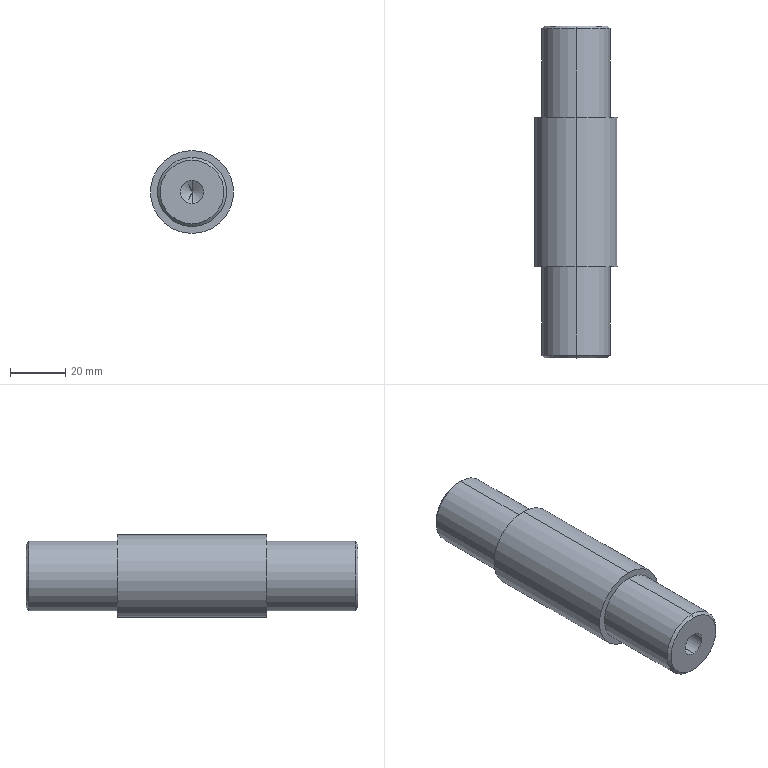Part | STEP file | PN_0023 | 1 solid | 22 faces | box 30 x 120 x 30 mm | volume 67614 mm3 | cylinder 10 | cone 8 | plane 4 | commonest cylinder face diameters 8.5 x4 25 x4 30 x2
STEP:
#1=CARTESIAN_POINT('',(0.,0.,0.));
#2=DIRECTION('',(0.,0.,1.));
#3=DIRECTION('',(1.,0.,0.));
#4=AXIS2_PLACEMENT_3D('',#1,#2,#3);
#5=CARTESIAN_POINT('',(0.,0.,-11.5));
#6=VERTEX_POINT('',#5);
#7=CARTESIAN_POINT('',(0.,0.,11.5));
#8=VERTEX_POINT('',#7);
#9=CARTESIAN_POINT('',(0.,0.,0.));
#10=DIRECTION('',(0.,-1.,0.));
#11=DIRECTION('',(0.,0.,-1.));
#12=AXIS2_PLACEMENT_3D('',#9,#10,#11);
#13=CIRCLE('',#12,11.5);
#14=CARTESIAN_POINT('',(0.,0.,0.));
#15=DIRECTION('',(0.,1.,0.));
#16=DIRECTION('',(0.,0.,1.));
#17=AXIS2_PLACEMENT_3D('',#14,#15,#16);
#18=CONICAL_SURFACE('',#17,11.5,0.7854);
#19=CARTESIAN_POINT('',(3.142,0.));
#20=DIRECTION('',(-1.,0.));
#21=VECTOR('',#20,1.);
#22=LINE('',#19,#21);
#23=(GEOMETRIC_REPRESENTATION_CONTEXT(2)PARAMETRIC_REPRESENTATION_CONTEXT()REPRESENTATION_CONTEXT('',''));
#24=DEFINITIONAL_REPRESENTATION('',(#22),#23);
#25=PCURVE('',#18,#24);
#26=CARTESIAN_POINT('',(0.,0.,0.));
#27=DIRECTION('',(0.,-1.,0.));
#28=DIRECTION('',(0.,0.,-1.));
#29=AXIS2_PLACEMENT_3D('',#26,#27,#28);
#30=PLANE('',#29);
#31=CARTESIAN_POINT('',(0.,0.));
#32=DIRECTION('',(1.,0.));
#33=AXIS2_PLACEMENT_2D('',#31,#32);
#34=CIRCLE('',#33,11.5);
#35=(GEOMETRIC_REPRESENTATION_CONTEXT(2)PARAMETRIC_REPRESENTATION_CONTEXT()REPRESENTATION_CONTEXT('',''));
#36=DEFINITIONAL_REPRESENTATION('',(#34),#35);
#37=PCURVE('',#30,#36);
#38=SURFACE_CURVE('',#13,(#25,#37),.PCURVE_S1.);
#39=EDGE_CURVE('',#6,#8,#38,.T.);
#40=ORIENTED_EDGE('',*,*,#39,.F.);
#41=CARTESIAN_POINT('',(0.,1.,-12.5));
#42=VERTEX_POINT('',#41);
#43=CARTESIAN_POINT('',(0.,0.,-11.5));
#44=DIRECTION('',(0.,0.7071,-0.7071));
#45=VECTOR('',#44,1.);
#46=LINE('',#43,#45);
#47=CARTESIAN_POINT('',(3.142,0.));
#48=DIRECTION('',(0.,1.));
#49=VECTOR('',#48,1.);
#50=LINE('',#47,#49);
#51=(GEOMETRIC_REPRESENTATION_CONTEXT(2)PARAMETRIC_REPRESENTATION_CONTEXT()REPRESENTATION_CONTEXT('',''));
#52=DEFINITIONAL_REPRESENTATION('',(#50),#51);
#53=PCURVE('',#18,#52);
#54=CARTESIAN_POINT('',(0.,0.,0.));
#55=DIRECTION('',(0.,1.,0.));
#56=DIRECTION('',(0.,0.,1.));
#57=AXIS2_PLACEMENT_3D('',#54,#55,#56);
#58=CONICAL_SURFACE('',#57,11.5,0.7854);
#59=CARTESIAN_POINT('',(3.142,0.));
#60=DIRECTION('',(0.,1.));
#61=VECTOR('',#60,1.);
#62=LINE('',#59,#61);
#63=(GEOMETRIC_REPRESENTATION_CONTEXT(2)PARAMETRIC_REPRESENTATION_CONTEXT()REPRESENTATION_CONTEXT('',''));
#64=DEFINITIONAL_REPRESENTATION('',(#62),#63);
#65=PCURVE('',#58,#64);
#66=SURFACE_CURVE('',#46,(#53,#65),.PCURVE_S1.);
#67=EDGE_CURVE('',#6,#42,#66,.T.);
#68=ORIENTED_EDGE('',*,*,#67,.T.);
#69=CARTESIAN_POINT('',(0.,1.,12.5));
#70=VERTEX_POINT('',#69);
#71=CARTESIAN_POINT('',(0.,1.,0.));
#72=DIRECTION('',(0.,1.,0.));
#73=DIRECTION('',(0.,0.,-1.));
#74=AXIS2_PLACEMENT_3D('',#71,#72,#73);
#75=CIRCLE('',#74,12.5);
#76=CARTESIAN_POINT('',(-3.142,1.));
#77=DIRECTION('',(1.,0.));
#78=VECTOR('',#77,1.);
#79=LINE('',#76,#78);
#80=(GEOMETRIC_REPRESENTATION_CONTEXT(2)PARAMETRIC_REPRESENTATION_CONTEXT()REPRESENTATION_CONTEXT('',''));
#81=DEFINITIONAL_REPRESENTATION('',(#79),#80);
#82=PCURVE('',#18,#81);
#83=CARTESIAN_POINT('',(0.,0.,0.));
#84=DIRECTION('',(0.,-1.,0.));
#85=DIRECTION('',(0.,0.,-1.));
#86=AXIS2_PLACEMENT_3D('',#83,#84,#85);
#87=CYLINDRICAL_SURFACE('',#86,12.5);
#88=CARTESIAN_POINT('',(6.283,-1.));
#89=DIRECTION('',(-1.,0.));
#90=VECTOR('',#89,1.);
#91=LINE('',#88,#90);
#92=(GEOMETRIC_REPRESENTATION_CONTEXT(2)PARAMETRIC_REPRESENTATION_CONTEXT()REPRESENTATION_CONTEXT('',''));
#93=DEFINITIONAL_REPRESENTATION('',(#91),#92);
#94=PCURVE('',#87,#93);
#95=SURFACE_CURVE('',#75,(#82,#94),.PCURVE_S1.);
#96=EDGE_CURVE('',#70,#42,#95,.T.);
#97=ORIENTED_EDGE('',*,*,#96,.F.);
#98=CARTESIAN_POINT('',(0.,0.,11.5));
#99=DIRECTION('',(0.,0.7071,0.7071));
#100=VECTOR('',#99,1.);
#101=LINE('',#98,#100);
#102=CARTESIAN_POINT('',(0.,0.));
#103=DIRECTION('',(0.,1.));
#104=VECTOR('',#103,1.);
#105=LINE('',#102,#104);
#106=(GEOMETRIC_REPRESENTATION_CONTEXT(2)PARAMETRIC_REPRESENTATION_CONTEXT()REPRESENTATION_CONTEXT('',''));
#107=DEFINITIONAL_REPRESENTATION('',(#105),#106);
#108=PCURVE('',#18,#107);
#109=CARTESIAN_POINT('',(6.283,0.));
#110=DIRECTION('',(0.,1.));
#111=VECTOR('',#110,1.);
#112=LINE('',#109,#111);
#113=(GEOMETRIC_REPRESENTATION_CONTEXT(2)PARAMETRIC_REPRESENTATION_CONTEXT()REPRESENTATION_CONTEXT('',''));
#114=DEFINITIONAL_REPRESENTATION('',(#112),#113);
#115=PCURVE('',#58,#114);
#116=SURFACE_CURVE('',#101,(#108,#115),.PCURVE_S1.);
#117=EDGE_CURVE('',#8,#70,#116,.T.);
#118=ORIENTED_EDGE('',*,*,#117,.F.);
#119=EDGE_LOOP('',(#40,#68,#97,#118));
#120=FACE_BOUND('',#119,.T.);
#121=ADVANCED_FACE('',(#120),#18,.T.);
#122=CARTESIAN_POINT('',(0.,120.,11.5));
#123=VERTEX_POINT('',#122);
#124=CARTESIAN_POINT('',(0.,120.,-11.5));
#125=VERTEX_POINT('',#124);
#126=CARTESIAN_POINT('',(0.,120.,0.));
#127=DIRECTION('',(0.,1.,0.));
#128=DIRECTION('',(0.,0.,1.));
#129=AXIS2_PLACEMENT_3D('',#126,#127,#128);
#130=CIRCLE('',#129,11.5);
#131=CARTESIAN_POINT('',(0.,119.,0.));
#132=DIRECTION('',(0.,-1.,0.));
#133=DIRECTION('',(0.,0.,-1.));
#134=AXIS2_PLACEMENT_3D('',#131,#132,#133);
#135=CONICAL_SURFACE('',#134,12.5,0.7854);
#136=CARTESIAN_POINT('',(3.142,-1.));
#137=DIRECTION('',(-1.,0.));
#138=VECTOR('',#137,1.);
#139=LINE('',#136,#138);
#140=(GEOMETRIC_REPRESENTATION_CONTEXT(2)PARAMETRIC_REPRESENTATION_CONTEXT()REPRESENTATION_CONTEXT('',''));
#141=DEFINITIONAL_REPRESENTATION('',(#139),#140);
#142=PCURVE('',#135,#141);
#143=CARTESIAN_POINT('',(0.,120.,0.));
#144=DIRECTION('',(0.,1.,0.));
#145=DIRECTION('',(0.,0.,1.));
#146=AXIS2_PLACEMENT_3D('',#143,#144,#145);
#147=PLANE('',#146);
#148=CARTESIAN_POINT('',(0.,0.));
#149=DIRECTION('',(1.,0.));
#150=AXIS2_PLACEMENT_2D('',#148,#149);
#151=CIRCLE('',#150,11.5);
#152=(GEOMETRIC_REPRESENTATION_CONTEXT(2)PARAMETRIC_REPRESENTATION_CONTEXT()REPRESENTATION_CONTEXT('',''));
#153=DEFINITIONAL_REPRESENTATION('',(#151),#152);
#154=PCURVE('',#147,#153);
#155=SURFACE_CURVE('',#130,(#142,#154),.PCURVE_S1.);
#156=EDGE_CURVE('',#123,#125,#155,.T.);
#157=ORIENTED_EDGE('',*,*,#156,.F.);
#158=CARTESIAN_POINT('',(0.,119.,12.5));
#159=VERTEX_POINT('',#158);
#160=CARTESIAN_POINT('',(0.,119.,12.5));
#161=DIRECTION('',(0.,-0.7071,0.7071));
#162=VECTOR('',#161,1.);
#163=LINE('',#160,#162);
#164=CARTESIAN_POINT('',(3.142,0.));
#165=DIRECTION('',(0.,1.));
#166=VECTOR('',#165,1.);
#167=LINE('',#164,#166);
#168=(GEOMETRIC_REPRESENTATION_CONTEXT(2)PARAMETRIC_REPRESENTATION_CONTEXT()REPRESENTATION_CONTEXT('',''));
#169=DEFINITIONAL_REPRESENTATION('',(#167),#168);
#170=PCURVE('',#135,#169);
#171=CARTESIAN_POINT('',(0.,119.,0.));
#172=DIRECTION('',(0.,-1.,0.));
#173=DIRECTION('',(0.,0.,-1.));
#174=AXIS2_PLACEMENT_3D('',#171,#172,#173);
#175=CONICAL_SURFACE('',#174,12.5,0.7854);
#176=CARTESIAN_POINT('',(3.142,0.));
#177=DIRECTION('',(0.,1.));
#178=VECTOR('',#177,1.);
#179=LINE('',#176,#178);
#180=(GEOMETRIC_REPRESENTATION_CONTEXT(2)PARAMETRIC_REPRESENTATION_CONTEXT()REPRESENTATION_CONTEXT('',''));
#181=DEFINITIONAL_REPRESENTATION('',(#179),#180);
#182=PCURVE('',#175,#181);
#183=SURFACE_CURVE('',#163,(#170,#182),.PCURVE_S1.);
#184=EDGE_CURVE('',#123,#159,#183,.T.);
#185=ORIENTED_EDGE('',*,*,#184,.T.);
#186=CARTESIAN_POINT('',(0.,119.,-12.5));
#187=VERTEX_POINT('',#186);
#188=CARTESIAN_POINT('',(0.,119.,0.));
#189=DIRECTION('',(0.,-1.,0.));
#190=DIRECTION('',(0.,0.,1.));
#191=AXIS2_PLACEMENT_3D('',#188,#189,#190);
#192=CIRCLE('',#191,12.5);
#193=CARTESIAN_POINT('',(-3.142,0.));
#194=DIRECTION('',(1.,0.));
#195=VECTOR('',#194,1.);
#196=LINE('',#193,#195);
#197=(GEOMETRIC_REPRESENTATION_CONTEXT(2)PARAMETRIC_REPRESENTATION_CONTEXT()REPRESENTATION_CONTEXT('',''));
#198=DEFINITIONAL_REPRESENTATION('',(#196),#197);
#199=PCURVE('',#135,#198);
#200=CARTESIAN_POINT('',(0.,0.,0.));
#201=DIRECTION('',(0.,-1.,0.));
#202=DIRECTION('',(0.,0.,-1.));
#203=AXIS2_PLACEMENT_3D('',#200,#201,#202);
#204=CYLINDRICAL_SURFACE('',#203,12.5);
#205=CARTESIAN_POINT('',(-3.142,-119.));
#206=DIRECTION('',(1.,0.));
#207=VECTOR('',#206,1.);
#208=LINE('',#205,#207);
#209=(GEOMETRIC_REPRESENTATION_CONTEXT(2)PARAMETRIC_REPRESENTATION_CONTEXT()REPRESENTATION_CONTEXT('',''));
#210=DEFINITIONAL_REPRESENTATION('',(#208),#209);
#211=PCURVE('',#204,#210);
#212=SURFACE_CURVE('',#192,(#199,#211),.PCURVE_S1.);
#213=EDGE_CURVE('',#187,#159,#212,.T.);
#214=ORIENTED_EDGE('',*,*,#213,.F.);
#215=CARTESIAN_POINT('',(0.,119.,-12.5));
#216=DIRECTION('',(0.,-0.7071,-0.7071));
#217=VECTOR('',#216,1.);
#218=LINE('',#215,#217);
#219=CARTESIAN_POINT('',(0.,0.));
#220=DIRECTION('',(0.,1.));
#221=VECTOR('',#220,1.);
#222=LINE('',#219,#221);
#223=(GEOMETRIC_REPRESENTATION_CONTEXT(2)PARAMETRIC_REPRESENTATION_CONTEXT()REPRESENTATION_CONTEXT('',''));
#224=DEFINITIONAL_REPRESENTATION('',(#222),#223);
#225=PCURVE('',#135,#224);
#226=CARTESIAN_POINT('',(6.283,0.));
#227=DIRECTION('',(0.,1.));
#228=VECTOR('',#227,1.);
#229=LINE('',#226,#228);
#230=(GEOMETRIC_REPRESENTATION_CONTEXT(2)PARAMETRIC_REPRESENTATION_CONTEXT()REPRESENTATION_CONTEXT('',''));
#231=DEFINITIONAL_REPRESENTATION('',(#229),#230);
#232=PCURVE('',#175,#231);
#233=SURFACE_CURVE('',#218,(#225,#232),.PCURVE_S1.);
#234=EDGE_CURVE('',#125,#187,#233,.T.);
#235=ORIENTED_EDGE('',*,*,#234,.F.);
#236=EDGE_LOOP('',(#157,#185,#214,#235));
#237=FACE_BOUND('',#236,.T.);
#238=ADVANCED_FACE('',(#237),#135,.T.);
#239=CARTESIAN_POINT('',(0.,24.5,-4.25));
#240=VERTEX_POINT('',#239);
#241=CARTESIAN_POINT('',(0.,0.,-4.25));
#242=VERTEX_POINT('',#241);
#243=CARTESIAN_POINT('',(0.,0.,-4.25));
#244=DIRECTION('',(0.,-1.,0.));
#245=VECTOR('',#244,1.);
#246=LINE('',#243,#245);
#247=CARTESIAN_POINT('',(0.,0.,0.));
#248=DIRECTION('',(0.,-1.,0.));
#249=DIRECTION('',(0.,0.,-1.));
#250=AXIS2_PLACEMENT_3D('',#247,#248,#249);
#251=CYLINDRICAL_SURFACE('',#250,4.25);
#252=CARTESIAN_POINT('',(6.283,0.));
#253=DIRECTION('',(0.,1.));
#254=VECTOR('',#253,1.);
#255=LINE('',#252,#254);
#256=(GEOMETRIC_REPRESENTATION_CONTEXT(2)PARAMETRIC_REPRESENTATION_CONTEXT()REPRESENTATION_CONTEXT('',''));
#257=DEFINITIONAL_REPRESENTATION('',(#255),#256);
#258=PCURVE('',#251,#257);
#259=CARTESIAN_POINT('',(0.,0.,0.));
#260=DIRECTION('',(0.,-1.,0.));
#261=DIRECTION('',(0.,0.,-1.));
#262=AXIS2_PLACEMENT_3D('',#259,#260,#261);
#263=CYLINDRICAL_SURFACE('',#262,4.25);
#264=CARTESIAN_POINT('',(0.,0.));
#265=DIRECTION('',(0.,1.));
#266=VECTOR('',#265,1.);
#267=LINE('',#264,#266);
#268=(GEOMETRIC_REPRESENTATION_CONTEXT(2)PARAMETRIC_REPRESENTATION_CONTEXT()REPRESENTATION_CONTEXT('',''));
#269=DEFINITIONAL_REPRESENTATION('',(#267),#268);
#270=PCURVE('',#263,#269);
#271=SURFACE_CURVE('',#246,(#258,#270),.PCURVE_S1.);
#272=EDGE_CURVE('',#240,#242,#271,.T.);
#273=ORIENTED_EDGE('',*,*,#272,.T.);
#274=CARTESIAN_POINT('',(0.,0.,4.25));
#275=VERTEX_POINT('',#274);
#276=CARTESIAN_POINT('',(0.,0.,0.));
#277=DIRECTION('',(0.,-1.,0.));
#278=DIRECTION('',(0.,0.,-1.));
#279=AXIS2_PLACEMENT_3D('',#276,#277,#278);
#280=CIRCLE('',#279,4.25);
#281=CARTESIAN_POINT('',(0.,0.));
#282=DIRECTION('',(1.,0.));
#283=VECTOR('',#282,1.);
#284=LINE('',#281,#283);
#285=(GEOMETRIC_REPRESENTATION_CONTEXT(2)PARAMETRIC_REPRESENTATION_CONTEXT()REPRESENTATION_CONTEXT('',''));
#286=DEFINITIONAL_REPRESENTATION('',(#284),#285);
#287=PCURVE('',#251,#286);
#288=CARTESIAN_POINT('',(0.,0.));
#289=DIRECTION('',(1.,0.));
#290=AXIS2_PLACEMENT_2D('',#288,#289);
#291=CIRCLE('',#290,4.25);
#292=(GEOMETRIC_REPRESENTATION_CONTEXT(2)PARAMETRIC_REPRESENTATION_CONTEXT()REPRESENTATION_CONTEXT('',''));
#293=DEFINITIONAL_REPRESENTATION('',(#291),#292);
#294=PCURVE('',#30,#293);
#295=SURFACE_CURVE('',#280,(#287,#294),.PCURVE_S1.);
#296=EDGE_CURVE('',#275,#242,#295,.T.);
#297=ORIENTED_EDGE('',*,*,#296,.F.);
#298=CARTESIAN_POINT('',(0.,24.5,4.25));
#299=VERTEX_POINT('',#298);
#300=CARTESIAN_POINT('',(0.,0.,4.25));
#301=DIRECTION('',(0.,-1.,0.));
#302=VECTOR('',#301,1.);
#303=LINE('',#300,#302);
#304=CARTESIAN_POINT('',(3.142,0.));
#305=DIRECTION('',(0.,1.));
#306=VECTOR('',#305,1.);
#307=LINE('',#304,#306);
#308=(GEOMETRIC_REPRESENTATION_CONTEXT(2)PARAMETRIC_REPRESENTATION_CONTEXT()REPRESENTATION_CONTEXT('',''));
#309=DEFINITIONAL_REPRESENTATION('',(#307),#308);
#310=PCURVE('',#251,#309);
#311=CARTESIAN_POINT('',(3.142,0.));
#312=DIRECTION('',(0.,1.));
#313=VECTOR('',#312,1.);
#314=LINE('',#311,#313);
#315=(GEOMETRIC_REPRESENTATION_CONTEXT(2)PARAMETRIC_REPRESENTATION_CONTEXT()REPRESENTATION_CONTEXT('',''));
#316=DEFINITIONAL_REPRESENTATION('',(#314),#315);
#317=PCURVE('',#263,#316);
#318=SURFACE_CURVE('',#303,(#310,#317),.PCURVE_S1.);
#319=EDGE_CURVE('',#299,#275,#318,.T.);
#320=ORIENTED_EDGE('',*,*,#319,.F.);
#321=CARTESIAN_POINT('',(0.,24.5,0.));
#322=DIRECTION('',(0.,-1.,0.));
#323=DIRECTION('',(0.,0.,-1.));
#324=AXIS2_PLACEMENT_3D('',#321,#322,#323);
#325=CIRCLE('',#324,4.25);
#326=CARTESIAN_POINT('',(0.,-24.5));
#327=DIRECTION('',(1.,0.));
#328=VECTOR('',#327,1.);
#329=LINE('',#326,#328);
#330=(GEOMETRIC_REPRESENTATION_CONTEXT(2)PARAMETRIC_REPRESENTATION_CONTEXT()REPRESENTATION_CONTEXT('',''));
#331=DEFINITIONAL_REPRESENTATION('',(#329),#330);
#332=PCURVE('',#251,#331);
#333=CARTESIAN_POINT('',(0.,24.5,0.));
#334=DIRECTION('',(0.,-1.,0.));
#335=DIRECTION('',(0.,0.,-1.));
#336=AXIS2_PLACEMENT_3D('',#333,#334,#335);
#337=CONICAL_SURFACE('',#336,4.25,1.03);
#338=CARTESIAN_POINT('',(0.,0.));
#339=DIRECTION('',(1.,0.));
#340=VECTOR('',#339,1.);
#341=LINE('',#338,#340);
#342=(GEOMETRIC_REPRESENTATION_CONTEXT(2)PARAMETRIC_REPRESENTATION_CONTEXT()REPRESENTATION_CONTEXT('',''));
#343=DEFINITIONAL_REPRESENTATION('',(#341),#342);
#344=PCURVE('',#337,#343);
#345=SURFACE_CURVE('',#325,(#332,#344),.PCURVE_S1.);
#346=EDGE_CURVE('',#299,#240,#345,.T.);
#347=ORIENTED_EDGE('',*,*,#346,.T.);
#348=EDGE_LOOP('',(#273,#297,#320,#347));
#349=FACE_BOUND('',#348,.F.);
#350=ADVANCED_FACE('',(#349),#251,.F.);
#351=ORIENTED_EDGE('',*,*,#346,.F.);
#352=CARTESIAN_POINT('',(0.,27.054,0.));
#353=VERTEX_POINT('',#352);
#354=CARTESIAN_POINT('',(0.,24.5,4.25));
#355=DIRECTION('',(0.,-0.515,0.8572));
#356=VECTOR('',#355,1.);
#357=LINE('',#354,#356);
#358=CARTESIAN_POINT('',(3.142,0.));
#359=DIRECTION('',(0.,1.));
#360=VECTOR('',#359,1.);
#361=LINE('',#358,#360);
#362=(GEOMETRIC_REPRESENTATION_CONTEXT(2)PARAMETRIC_REPRESENTATION_CONTEXT()REPRESENTATION_CONTEXT('',''));
#363=DEFINITIONAL_REPRESENTATION('',(#361),#362);
#364=PCURVE('',#337,#363);
#365=CARTESIAN_POINT('',(0.,24.5,0.));
#366=DIRECTION('',(0.,-1.,0.));
#367=DIRECTION('',(0.,0.,-1.));
#368=AXIS2_PLACEMENT_3D('',#365,#366,#367);
#369=CONICAL_SURFACE('',#368,4.25,1.03);
#370=CARTESIAN_POINT('',(3.142,0.));
#371=DIRECTION('',(0.,1.));
#372=VECTOR('',#371,1.);
#373=LINE('',#370,#372);
#374=(GEOMETRIC_REPRESENTATION_CONTEXT(2)PARAMETRIC_REPRESENTATION_CONTEXT()REPRESENTATION_CONTEXT('',''));
#375=DEFINITIONAL_REPRESENTATION('',(#373),#374);
#376=PCURVE('',#369,#375);
#377=SURFACE_CURVE('',#357,(#364,#376),.PCURVE_S1.);
#378=EDGE_CURVE('',#353,#299,#377,.T.);
#379=ORIENTED_EDGE('',*,*,#378,.F.);
#380=CARTESIAN_POINT('',(0.,24.5,-4.25));
#381=DIRECTION('',(0.,-0.515,-0.8572));
#382=VECTOR('',#381,1.);
#383=LINE('',#380,#382);
#384=CARTESIAN_POINT('',(6.283,0.));
#385=DIRECTION('',(0.,1.));
#386=VECTOR('',#385,1.);
#387=LINE('',#384,#386);
#388=(GEOMETRIC_REPRESENTATION_CONTEXT(2)PARAMETRIC_REPRESENTATION_CONTEXT()REPRESENTATION_CONTEXT('',''));
#389=DEFINITIONAL_REPRESENTATION('',(#387),#388);
#390=PCURVE('',#337,#389);
#391=CARTESIAN_POINT('',(0.,0.));
#392=DIRECTION('',(0.,1.));
#393=VECTOR('',#392,1.);
#394=LINE('',#391,#393);
#395=(GEOMETRIC_REPRESENTATION_CONTEXT(2)PARAMETRIC_REPRESENTATION_CONTEXT()REPRESENTATION_CONTEXT('',''));
#396=DEFINITIONAL_REPRESENTATION('',(#394),#395);
#397=PCURVE('',#369,#396);
#398=SURFACE_CURVE('',#383,(#390,#397),.PCURVE_S1.);
#399=EDGE_CURVE('',#353,#240,#398,.T.);
#400=ORIENTED_EDGE('',*,*,#399,.T.);
#401=EDGE_LOOP('',(#351,#379,#400));
#402=FACE_BOUND('',#401,.F.);
#403=ADVANCED_FACE('',(#402),#337,.F.);
#404=CARTESIAN_POINT('',(-0.002204,95.5,4.252));
#405=VERTEX_POINT('',#404);
#406=CARTESIAN_POINT('',(-0.002204,120.,4.252));
#407=VERTEX_POINT('',#406);
#408=CARTESIAN_POINT('',(-0.002204,120.,4.252));
#409=DIRECTION('',(0.,1.,0.));
#410=VECTOR('',#409,1.);
#411=LINE('',#408,#410);
#412=CARTESIAN_POINT('',(-0.002204,120.,0.001923));
#413=DIRECTION('',(0.,1.,0.));
#414=DIRECTION('',(0.,0.,1.));
#415=AXIS2_PLACEMENT_3D('',#412,#413,#414);
#416=CYLINDRICAL_SURFACE('',#415,4.25);
#417=CARTESIAN_POINT('',(6.283,0.));
#418=DIRECTION('',(0.,1.));
#419=VECTOR('',#418,1.);
#420=LINE('',#417,#419);
#421=(GEOMETRIC_REPRESENTATION_CONTEXT(2)PARAMETRIC_REPRESENTATION_CONTEXT()REPRESENTATION_CONTEXT('',''));
#422=DEFINITIONAL_REPRESENTATION('',(#420),#421);
#423=PCURVE('',#416,#422);
#424=CARTESIAN_POINT('',(-0.002204,120.,0.001923));
#425=DIRECTION('',(0.,1.,0.));
#426=DIRECTION('',(0.,0.,1.));
#427=AXIS2_PLACEMENT_3D('',#424,#425,#426);
#428=CYLINDRICAL_SURFACE('',#427,4.25);
#429=CARTESIAN_POINT('',(0.,0.));
#430=DIRECTION('',(0.,1.));
#431=VECTOR('',#430,1.);
#432=LINE('',#429,#431);
#433=(GEOMETRIC_REPRESENTATION_CONTEXT(2)PARAMETRIC_REPRESENTATION_CONTEXT()REPRESENTATION_CONTEXT('',''));
#434=DEFINITIONAL_REPRESENTATION('',(#432),#433);
#435=PCURVE('',#428,#434);
#436=SURFACE_CURVE('',#411,(#423,#435),.PCURVE_S1.);
#437=EDGE_CURVE('',#405,#407,#436,.T.);
#438=ORIENTED_EDGE('',*,*,#437,.T.);
#439=CARTESIAN_POINT('',(-0.002204,120.,-4.248));
#440=VERTEX_POINT('',#439);
#441=CARTESIAN_POINT('',(-0.002204,120.,0.001923));
#442=DIRECTION('',(0.,1.,0.));
#443=DIRECTION('',(0.,0.,1.));
#444=AXIS2_PLACEMENT_3D('',#441,#442,#443);
#445=CIRCLE('',#444,4.25);
#446=CARTESIAN_POINT('',(0.,0.));
#447=DIRECTION('',(1.,0.));
#448=VECTOR('',#447,1.);
#449=LINE('',#446,#448);
#450=(GEOMETRIC_REPRESENTATION_CONTEXT(2)PARAMETRIC_REPRESENTATION_CONTEXT()REPRESENTATION_CONTEXT('',''));
#451=DEFINITIONAL_REPRESENTATION('',(#449),#450);
#452=PCURVE('',#416,#451);
#453=CARTESIAN_POINT('',(0.001923,-0.002204));
#454=DIRECTION('',(1.,0.));
#455=AXIS2_PLACEMENT_2D('',#453,#454);
#456=CIRCLE('',#455,4.25);
#457=(GEOMETRIC_REPRESENTATION_CONTEXT(2)PARAMETRIC_REPRESENTATION_CONTEXT()REPRESENTATION_CONTEXT('',''));
#458=DEFINITIONAL_REPRESENTATION('',(#456),#457);
#459=PCURVE('',#147,#458);
#460=SURFACE_CURVE('',#445,(#452,#459),.PCURVE_S1.);
#461=EDGE_CURVE('',#440,#407,#460,.T.);
#462=ORIENTED_EDGE('',*,*,#461,.F.);
#463=CARTESIAN_POINT('',(-0.002204,95.5,-4.248));
#464=VERTEX_POINT('',#463);
#465=CARTESIAN_POINT('',(-0.002204,120.,-4.248));
#466=DIRECTION('',(0.,1.,0.));
#467=VECTOR('',#466,1.);
#468=LINE('',#465,#467);
#469=CARTESIAN_POINT('',(3.142,0.));
#470=DIRECTION('',(0.,1.));
#471=VECTOR('',#470,1.);
#472=LINE('',#469,#471);
#473=(GEOMETRIC_REPRESENTATION_CONTEXT(2)PARAMETRIC_REPRESENTATION_CONTEXT()REPRESENTATION_CONTEXT('',''));
#474=DEFINITIONAL_REPRESENTATION('',(#472),#473);
#475=PCURVE('',#416,#474);
#476=CARTESIAN_POINT('',(3.142,0.));
#477=DIRECTION('',(0.,1.));
#478=VECTOR('',#477,1.);
#479=LINE('',#476,#478);
#480=(GEOMETRIC_REPRESENTATION_CONTEXT(2)PARAMETRIC_REPRESENTATION_CONTEXT()REPRESENTATION_CONTEXT('',''));
#481=DEFINITIONAL_REPRESENTATION('',(#479),#480);
#482=PCURVE('',#428,#481);
#483=SURFACE_CURVE('',#468,(#475,#482),.PCURVE_S1.);
#484=EDGE_CURVE('',#464,#440,#483,.T.);
#485=ORIENTED_EDGE('',*,*,#484,.F.);
#486=CARTESIAN_POINT('',(-0.002204,95.5,0.001923));
#487=DIRECTION('',(0.,1.,0.));
#488=DIRECTION('',(0.,0.,1.));
#489=AXIS2_PLACEMENT_3D('',#486,#487,#488);
#490=CIRCLE('',#489,4.25);
#491=CARTESIAN_POINT('',(0.,-24.5));
#492=DIRECTION('',(1.,0.));
#493=VECTOR('',#492,1.);
#494=LINE('',#491,#493);
#495=(GEOMETRIC_REPRESENTATION_CONTEXT(2)PARAMETRIC_REPRESENTATION_CONTEXT()REPRESENTATION_CONTEXT('',''));
#496=DEFINITIONAL_REPRESENTATION('',(#494),#495);
#497=PCURVE('',#416,#496);
#498=CARTESIAN_POINT('',(-0.002204,95.5,0.001923));
#499=DIRECTION('',(0.,1.,0.));
#500=DIRECTION('',(0.,0.,1.));
#501=AXIS2_PLACEMENT_3D('',#498,#499,#500);
#502=CONICAL_SURFACE('',#501,4.25,1.03);
#503=CARTESIAN_POINT('',(0.,0.));
#504=DIRECTION('',(1.,0.));
#505=VECTOR('',#504,1.);
#506=LINE('',#503,#505);
#507=(GEOMETRIC_REPRESENTATION_CONTEXT(2)PARAMETRIC_REPRESENTATION_CONTEXT()REPRESENTATION_CONTEXT('',''));
#508=DEFINITIONAL_REPRESENTATION('',(#506),#507);
#509=PCURVE('',#502,#508);
#510=SURFACE_CURVE('',#490,(#497,#509),.PCURVE_S1.);
#511=EDGE_CURVE('',#464,#405,#510,.T.);
#512=ORIENTED_EDGE('',*,*,#511,.T.);
#513=EDGE_LOOP('',(#438,#462,#485,#512));
#514=FACE_BOUND('',#513,.F.);
#515=ADVANCED_FACE('',(#514),#416,.F.);
#516=ORIENTED_EDGE('',*,*,#511,.F.);
#517=CARTESIAN_POINT('',(-0.002204,92.946,0.001923));
#518=VERTEX_POINT('',#517);
#519=CARTESIAN_POINT('',(-0.002204,95.5,-4.248));
#520=DIRECTION('',(0.,0.515,-0.8572));
#521=VECTOR('',#520,1.);
#522=LINE('',#519,#521);
#523=CARTESIAN_POINT('',(3.142,0.));
#524=DIRECTION('',(0.,1.));
#525=VECTOR('',#524,1.);
#526=LINE('',#523,#525);
#527=(GEOMETRIC_REPRESENTATION_CONTEXT(2)PARAMETRIC_REPRESENTATION_CONTEXT()REPRESENTATION_CONTEXT('',''));
#528=DEFINITIONAL_REPRESENTATION('',(#526),#527);
#529=PCURVE('',#502,#528);
#530=CARTESIAN_POINT('',(-0.002204,95.5,0.001923));
#531=DIRECTION('',(0.,1.,0.));
#532=DIRECTION('',(0.,0.,1.));
#533=AXIS2_PLACEMENT_3D('',#530,#531,#532);
#534=CONICAL_SURFACE('',#533,4.25,1.03);
#535=CARTESIAN_POINT('',(3.142,0.));
#536=DIRECTION('',(0.,1.));
#537=VECTOR('',#536,1.);
#538=LINE('',#535,#537);
#539=(GEOMETRIC_REPRESENTATION_CONTEXT(2)PARAMETRIC_REPRESENTATION_CONTEXT()REPRESENTATION_CONTEXT('',''));
#540=DEFINITIONAL_REPRESENTATION('',(#538),#539);
#541=PCURVE('',#534,#540);
#542=SURFACE_CURVE('',#522,(#529,#541),.PCURVE_S1.);
#543=EDGE_CURVE('',#518,#464,#542,.T.);
#544=ORIENTED_EDGE('',*,*,#543,.F.);
#545=CARTESIAN_POINT('',(-0.002204,95.5,4.252));
#546=DIRECTION('',(0.,0.515,0.8572));
#547=VECTOR('',#546,1.);
#548=LINE('',#545,#547);
#549=CARTESIAN_POINT('',(6.283,0.));
#550=DIRECTION('',(0.,1.));
#551=VECTOR('',#550,1.);
#552=LINE('',#549,#551);
#553=(GEOMETRIC_REPRESENTATION_CONTEXT(2)PARAMETRIC_REPRESENTATION_CONTEXT()REPRESENTATION_CONTEXT('',''));
#554=DEFINITIONAL_REPRESENTATION('',(#552),#553);
#555=PCURVE('',#502,#554);
#556=CARTESIAN_POINT('',(0.,0.));
#557=DIRECTION('',(0.,1.));
#558=VECTOR('',#557,1.);
#559=LINE('',#556,#558);
#560=(GEOMETRIC_REPRESENTATION_CONTEXT(2)PARAMETRIC_REPRESENTATION_CONTEXT()REPRESENTATION_CONTEXT('',''));
#561=DEFINITIONAL_REPRESENTATION('',(#559),#560);
#562=PCURVE('',#534,#561);
#563=SURFACE_CURVE('',#548,(#555,#562),.PCURVE_S1.);
#564=EDGE_CURVE('',#518,#405,#563,.T.);
#565=ORIENTED_EDGE('',*,*,#564,.T.);
#566=EDGE_LOOP('',(#516,#544,#565));
#567=FACE_BOUND('',#566,.F.);
#568=ADVANCED_FACE('',(#567),#502,.F.);
#569=CARTESIAN_POINT('',(0.,33.,-12.5));
#570=VERTEX_POINT('',#569);
#571=CARTESIAN_POINT('',(0.,33.,12.5));
#572=VERTEX_POINT('',#571);
#573=CARTESIAN_POINT('',(0.,33.,0.));
#574=DIRECTION('',(0.,-1.,0.));
#575=DIRECTION('',(0.,0.,-1.));
#576=AXIS2_PLACEMENT_3D('',#573,#574,#575);
#577=CIRCLE('',#576,12.5);
#578=CARTESIAN_POINT('',(0.,-33.));
#579=DIRECTION('',(1.,0.));
#580=VECTOR('',#579,1.);
#581=LINE('',#578,#580);
#582=(GEOMETRIC_REPRESENTATION_CONTEXT(2)PARAMETRIC_REPRESENTATION_CONTEXT()REPRESENTATION_CONTEXT('',''));
#583=DEFINITIONAL_REPRESENTATION('',(#581),#582);
#584=PCURVE('',#87,#583);
#585=CARTESIAN_POINT('',(12.5,33.,0.));
#586=DIRECTION('',(0.,-1.,0.));
#587=DIRECTION('',(0.,0.,-1.));
#588=AXIS2_PLACEMENT_3D('',#585,#586,#587);
#589=PLANE('',#588);
#590=CARTESIAN_POINT('',(0.,-12.5));
#591=DIRECTION('',(1.,0.));
#592=AXIS2_PLACEMENT_2D('',#590,#591);
#593=CIRCLE('',#592,12.5);
#594=(GEOMETRIC_REPRESENTATION_CONTEXT(2)PARAMETRIC_REPRESENTATION_CONTEXT()REPRESENTATION_CONTEXT('',''));
#595=DEFINITIONAL_REPRESENTATION('',(#593),#594);
#596=PCURVE('',#589,#595);
#597=SURFACE_CURVE('',#577,(#584,#596),.PCURVE_S1.);
#598=EDGE_CURVE('',#570,#572,#597,.T.);
#599=ORIENTED_EDGE('',*,*,#598,.T.);
#600=CARTESIAN_POINT('',(0.,0.,12.5));
#601=DIRECTION('',(0.,-1.,0.));
#602=VECTOR('',#601,1.);
#603=LINE('',#600,#602);
#604=CARTESIAN_POINT('',(3.142,0.));
#605=DIRECTION('',(0.,1.));
#606=VECTOR('',#605,1.);
#607=LINE('',#604,#606);
#608=(GEOMETRIC_REPRESENTATION_CONTEXT(2)PARAMETRIC_REPRESENTATION_CONTEXT()REPRESENTATION_CONTEXT('',''));
#609=DEFINITIONAL_REPRESENTATION('',(#607),#608);
#610=PCURVE('',#87,#609);
#611=CARTESIAN_POINT('',(0.,0.,0.));
#612=DIRECTION('',(0.,-1.,0.));
#613=DIRECTION('',(0.,0.,-1.));
#614=AXIS2_PLACEMENT_3D('',#611,#612,#613);
#615=CYLINDRICAL_SURFACE('',#614,12.5);
#616=CARTESIAN_POINT('',(3.142,0.));
#617=DIRECTION('',(0.,1.));
#618=VECTOR('',#617,1.);
#619=LINE('',#616,#618);
#620=(GEOMETRIC_REPRESENTATION_CONTEXT(2)PARAMETRIC_REPRESENTATION_CONTEXT()REPRESENTATION_CONTEXT('',''));
#621=DEFINITIONAL_REPRESENTATION('',(#619),#620);
#622=PCURVE('',#615,#621);
#623=SURFACE_CURVE('',#603,(#610,#622),.PCURVE_S1.);
#624=EDGE_CURVE('',#572,#70,#623,.T.);
#625=ORIENTED_EDGE('',*,*,#624,.T.);
#626=ORIENTED_EDGE('',*,*,#96,.T.);
#627=CARTESIAN_POINT('',(0.,0.,-12.5));
#628=DIRECTION('',(0.,-1.,0.));
#629=VECTOR('',#628,1.);
#630=LINE('',#627,#629);
#631=CARTESIAN_POINT('',(0.,0.));
#632=DIRECTION('',(0.,1.));
#633=VECTOR('',#632,1.);
#634=LINE('',#631,#633);
#635=(GEOMETRIC_REPRESENTATION_CONTEXT(2)PARAMETRIC_REPRESENTATION_CONTEXT()REPRESENTATION_CONTEXT('',''));
#636=DEFINITIONAL_REPRESENTATION('',(#634),#635);
#637=PCURVE('',#87,#636);
#638=CARTESIAN_POINT('',(6.283,0.));
#639=DIRECTION('',(0.,1.));
#640=VECTOR('',#639,1.);
#641=LINE('',#638,#640);
#642=(GEOMETRIC_REPRESENTATION_CONTEXT(2)PARAMETRIC_REPRESENTATION_CONTEXT()REPRESENTATION_CONTEXT('',''));
#643=DEFINITIONAL_REPRESENTATION('',(#641),#642);
#644=PCURVE('',#615,#643);
#645=SURFACE_CURVE('',#630,(#637,#644),.PCURVE_S1.);
#646=EDGE_CURVE('',#570,#42,#645,.T.);
#647=ORIENTED_EDGE('',*,*,#646,.F.);
#648=EDGE_LOOP('',(#599,#625,#626,#647));
#649=FACE_BOUND('',#648,.T.);
#650=ADVANCED_FACE('',(#649),#87,.T.);
#651=CARTESIAN_POINT('',(0.,87.,-15.));
#652=VERTEX_POINT('',#651);
#653=CARTESIAN_POINT('',(0.,87.,15.));
#654=VERTEX_POINT('',#653);
#655=CARTESIAN_POINT('',(0.,87.,0.));
#656=DIRECTION('',(0.,-1.,0.));
#657=DIRECTION('',(0.,0.,-1.));
#658=AXIS2_PLACEMENT_3D('',#655,#656,#657);
#659=CIRCLE('',#658,15.);
#660=CARTESIAN_POINT('',(0.,0.,0.));
#661=DIRECTION('',(0.,-1.,0.));
#662=DIRECTION('',(0.,0.,-1.));
#663=AXIS2_PLACEMENT_3D('',#660,#661,#662);
#664=CYLINDRICAL_SURFACE('',#663,15.);
#665=CARTESIAN_POINT('',(0.,-87.));
#666=DIRECTION('',(1.,0.));
#667=VECTOR('',#666,1.);
#668=LINE('',#665,#667);
#669=(GEOMETRIC_REPRESENTATION_CONTEXT(2)PARAMETRIC_REPRESENTATION_CONTEXT()REPRESENTATION_CONTEXT('',''));
#670=DEFINITIONAL_REPRESENTATION('',(#668),#669);
#671=PCURVE('',#664,#670);
#672=CARTESIAN_POINT('',(12.5,87.,0.));
#673=DIRECTION('',(0.,1.,0.));
#674=DIRECTION('',(0.,0.,1.));
#675=AXIS2_PLACEMENT_3D('',#672,#673,#674);
#676=PLANE('',#675);
#677=CARTESIAN_POINT('',(-15.,-12.5));
#678=CARTESIAN_POINT('',(-15.,13.481));
#679=CARTESIAN_POINT('',(7.5,0.4904));
#680=CARTESIAN_POINT('',(30.,-12.5));
#681=CARTESIAN_POINT('',(7.5,-25.49));
#682=CARTESIAN_POINT('',(-15.,-38.481));
#683=CARTESIAN_POINT('',(-15.,-12.5));
#684=(BOUNDED_CURVE()B_SPLINE_CURVE(2,(#677,#678,#679,#680,#681,#682,#683),.UNSPECIFIED.,.T.,.F.)B_SPLINE_CURVE_WITH_KNOTS((1,2,2,2,2,1),(-2.094,0.,2.094,4.189,6.283,8.378),.UNSPECIFIED.)CURVE()GEOMETRIC_REPRESENTATION_ITEM()RATIONAL_B_SPLINE_CURVE((1.,0.5,1.,0.5,1.,0.5,1.))REPRESENTATION_ITEM(''));
#685=(GEOMETRIC_REPRESENTATION_CONTEXT(2)PARAMETRIC_REPRESENTATION_CONTEXT()REPRESENTATION_CONTEXT('',''));
#686=DEFINITIONAL_REPRESENTATION('',(#684),#685);
#687=PCURVE('',#676,#686);
#688=SURFACE_CURVE('',#659,(#671,#687),.PCURVE_S1.);
#689=EDGE_CURVE('',#652,#654,#688,.T.);
#690=ORIENTED_EDGE('',*,*,#689,.T.);
#691=CARTESIAN_POINT('',(0.,33.,15.));
#692=VERTEX_POINT('',#691);
#693=CARTESIAN_POINT('',(0.,0.,15.));
#694=DIRECTION('',(0.,-1.,0.));
#695=VECTOR('',#694,1.);
#696=LINE('',#693,#695);
#697=CARTESIAN_POINT('',(3.142,0.));
#698=DIRECTION('',(0.,1.));
#699=VECTOR('',#698,1.);
#700=LINE('',#697,#699);
#701=(GEOMETRIC_REPRESENTATION_CONTEXT(2)PARAMETRIC_REPRESENTATION_CONTEXT()REPRESENTATION_CONTEXT('',''));
#702=DEFINITIONAL_REPRESENTATION('',(#700),#701);
#703=PCURVE('',#664,#702);
#704=CARTESIAN_POINT('',(0.,0.,0.));
#705=DIRECTION('',(0.,-1.,0.));
#706=DIRECTION('',(0.,0.,-1.));
#707=AXIS2_PLACEMENT_3D('',#704,#705,#706);
#708=CYLINDRICAL_SURFACE('',#707,15.);
#709=CARTESIAN_POINT('',(3.142,0.));
#710=DIRECTION('',(0.,1.));
#711=VECTOR('',#710,1.);
#712=LINE('',#709,#711);
#713=(GEOMETRIC_REPRESENTATION_CONTEXT(2)PARAMETRIC_REPRESENTATION_CONTEXT()REPRESENTATION_CONTEXT('',''));
#714=DEFINITIONAL_REPRESENTATION('',(#712),#713);
#715=PCURVE('',#708,#714);
#716=SURFACE_CURVE('',#696,(#703,#715),.PCURVE_S1.);
#717=EDGE_CURVE('',#654,#692,#716,.T.);
#718=ORIENTED_EDGE('',*,*,#717,.T.);
#719=CARTESIAN_POINT('',(0.,33.,-15.));
#720=VERTEX_POINT('',#719);
#721=CARTESIAN_POINT('',(0.,33.,0.));
#722=DIRECTION('',(0.,-1.,0.));
#723=DIRECTION('',(0.,0.,-1.));
#724=AXIS2_PLACEMENT_3D('',#721,#722,#723);
#725=CIRCLE('',#724,15.);
#726=CARTESIAN_POINT('',(0.,-33.));
#727=DIRECTION('',(1.,0.));
#728=VECTOR('',#727,1.);
#729=LINE('',#726,#728);
#730=(GEOMETRIC_REPRESENTATION_CONTEXT(2)PARAMETRIC_REPRESENTATION_CONTEXT()REPRESENTATION_CONTEXT('',''));
#731=DEFINITIONAL_REPRESENTATION('',(#729),#730);
#732=PCURVE('',#664,#731);
#733=CARTESIAN_POINT('',(0.,-12.5));
#734=DIRECTION('',(1.,0.));
#735=AXIS2_PLACEMENT_2D('',#733,#734);
#736=CIRCLE('',#735,15.);
#737=(GEOMETRIC_REPRESENTATION_CONTEXT(2)PARAMETRIC_REPRESENTATION_CONTEXT()REPRESENTATION_CONTEXT('',''));
#738=DEFINITIONAL_REPRESENTATION('',(#736),#737);
#739=PCURVE('',#589,#738);
#740=SURFACE_CURVE('',#725,(#732,#739),.PCURVE_S1.);
#741=EDGE_CURVE('',#720,#692,#740,.T.);
#742=ORIENTED_EDGE('',*,*,#741,.F.);
#743=CARTESIAN_POINT('',(0.,0.,-15.));
#744=DIRECTION('',(0.,-1.,0.));
#745=VECTOR('',#744,1.);
#746=LINE('',#743,#745);
#747=CARTESIAN_POINT('',(0.,0.));
#748=DIRECTION('',(0.,1.));
#749=VECTOR('',#748,1.);
#750=LINE('',#747,#749);
#751=(GEOMETRIC_REPRESENTATION_CONTEXT(2)PARAMETRIC_REPRESENTATION_CONTEXT()REPRESENTATION_CONTEXT('',''));
#752=DEFINITIONAL_REPRESENTATION('',(#750),#751);
#753=PCURVE('',#664,#752);
#754=CARTESIAN_POINT('',(6.283,0.));
#755=DIRECTION('',(0.,1.));
#756=VECTOR('',#755,1.);
#757=LINE('',#754,#756);
#758=(GEOMETRIC_REPRESENTATION_CONTEXT(2)PARAMETRIC_REPRESENTATION_CONTEXT()REPRESENTATION_CONTEXT('',''));
#759=DEFINITIONAL_REPRESENTATION('',(#757),#758);
#760=PCURVE('',#708,#759);
#761=SURFACE_CURVE('',#746,(#753,#760),.PCURVE_S1.);
#762=EDGE_CURVE('',#652,#720,#761,.T.);
#763=ORIENTED_EDGE('',*,*,#762,.F.);
#764=EDGE_LOOP('',(#690,#718,#742,#763));
#765=FACE_BOUND('',#764,.T.);
#766=ADVANCED_FACE('',(#765),#664,.T.);
#767=ORIENTED_EDGE('',*,*,#213,.T.);
#768=CARTESIAN_POINT('',(0.,87.,12.5));
#769=VERTEX_POINT('',#768);
#770=CARTESIAN_POINT('',(0.,0.,12.5));
#771=DIRECTION('',(0.,-1.,0.));
#772=VECTOR('',#771,1.);
#773=LINE('',#770,#772);
#774=CARTESIAN_POINT('',(3.142,0.));
#775=DIRECTION('',(0.,1.));
#776=VECTOR('',#775,1.);
#777=LINE('',#774,#776);
#778=(GEOMETRIC_REPRESENTATION_CONTEXT(2)PARAMETRIC_REPRESENTATION_CONTEXT()REPRESENTATION_CONTEXT('',''));
#779=DEFINITIONAL_REPRESENTATION('',(#777),#778);
#780=PCURVE('',#204,#779);
#781=CARTESIAN_POINT('',(0.,0.,0.));
#782=DIRECTION('',(0.,-1.,0.));
#783=DIRECTION('',(0.,0.,-1.));
#784=AXIS2_PLACEMENT_3D('',#781,#782,#783);
#785=CYLINDRICAL_SURFACE('',#784,12.5);
#786=CARTESIAN_POINT('',(3.142,0.));
#787=DIRECTION('',(0.,1.));
#788=VECTOR('',#787,1.);
#789=LINE('',#786,#788);
#790=(GEOMETRIC_REPRESENTATION_CONTEXT(2)PARAMETRIC_REPRESENTATION_CONTEXT()REPRESENTATION_CONTEXT('',''));
#791=DEFINITIONAL_REPRESENTATION('',(#789),#790);
#792=PCURVE('',#785,#791);
#793=SURFACE_CURVE('',#773,(#780,#792),.PCURVE_S1.);
#794=EDGE_CURVE('',#159,#769,#793,.T.);
#795=ORIENTED_EDGE('',*,*,#794,.T.);
#796=CARTESIAN_POINT('',(0.,87.,-12.5));
#797=VERTEX_POINT('',#796);
#798=CARTESIAN_POINT('',(0.,87.,0.));
#799=DIRECTION('',(0.,-1.,0.));
#800=DIRECTION('',(0.,0.,-1.));
#801=AXIS2_PLACEMENT_3D('',#798,#799,#800);
#802=CIRCLE('',#801,12.5);
#803=CARTESIAN_POINT('',(0.,-87.));
#804=DIRECTION('',(1.,0.));
#805=VECTOR('',#804,1.);
#806=LINE('',#803,#805);
#807=(GEOMETRIC_REPRESENTATION_CONTEXT(2)PARAMETRIC_REPRESENTATION_CONTEXT()REPRESENTATION_CONTEXT('',''));
#808=DEFINITIONAL_REPRESENTATION('',(#806),#807);
#809=PCURVE('',#204,#808);
#810=CARTESIAN_POINT('',(-12.5,-12.5));
#811=CARTESIAN_POINT('',(-12.5,9.151));
#812=CARTESIAN_POINT('',(6.25,-1.675));
#813=CARTESIAN_POINT('',(25.,-12.5));
#814=CARTESIAN_POINT('',(6.25,-23.325));
#815=CARTESIAN_POINT('',(-12.5,-34.151));
#816=CARTESIAN_POINT('',(-12.5,-12.5));
#817=(BOUNDED_CURVE()B_SPLINE_CURVE(2,(#810,#811,#812,#813,#814,#815,#816),.UNSPECIFIED.,.T.,.F.)B_SPLINE_CURVE_WITH_KNOTS((1,2,2,2,2,1),(-2.094,0.,2.094,4.189,6.283,8.378),.UNSPECIFIED.)CURVE()GEOMETRIC_REPRESENTATION_ITEM()RATIONAL_B_SPLINE_CURVE((1.,0.5,1.,0.5,1.,0.5,1.))REPRESENTATION_ITEM(''));
#818=(GEOMETRIC_REPRESENTATION_CONTEXT(2)PARAMETRIC_REPRESENTATION_CONTEXT()REPRESENTATION_CONTEXT('',''));
#819=DEFINITIONAL_REPRESENTATION('',(#817),#818);
#820=PCURVE('',#676,#819);
#821=SURFACE_CURVE('',#802,(#809,#820),.PCURVE_S1.);
#822=EDGE_CURVE('',#797,#769,#821,.T.);
#823=ORIENTED_EDGE('',*,*,#822,.F.);
#824=CARTESIAN_POINT('',(0.,0.,-12.5));
#825=DIRECTION('',(0.,-1.,0.));
#826=VECTOR('',#825,1.);
#827=LINE('',#824,#826);
#828=CARTESIAN_POINT('',(0.,0.));
#829=DIRECTION('',(0.,1.));
#830=VECTOR('',#829,1.);
#831=LINE('',#828,#830);
#832=(GEOMETRIC_REPRESENTATION_CONTEXT(2)PARAMETRIC_REPRESENTATION_CONTEXT()REPRESENTATION_CONTEXT('',''));
#833=DEFINITIONAL_REPRESENTATION('',(#831),#832);
#834=PCURVE('',#204,#833);
#835=CARTESIAN_POINT('',(6.283,0.));
#836=DIRECTION('',(0.,1.));
#837=VECTOR('',#836,1.);
#838=LINE('',#835,#837);
#839=(GEOMETRIC_REPRESENTATION_CONTEXT(2)PARAMETRIC_REPRESENTATION_CONTEXT()REPRESENTATION_CONTEXT('',''));
#840=DEFINITIONAL_REPRESENTATION('',(#838),#839);
#841=PCURVE('',#785,#840);
#842=SURFACE_CURVE('',#827,(#834,#841),.PCURVE_S1.);
#843=EDGE_CURVE('',#187,#797,#842,.T.);
#844=ORIENTED_EDGE('',*,*,#843,.F.);
#845=EDGE_LOOP('',(#767,#795,#823,#844));
#846=FACE_BOUND('',#845,.T.);
#847=ADVANCED_FACE('',(#846),#204,.T.);
#848=CARTESIAN_POINT('',(0.,120.,0.));
#849=DIRECTION('',(0.,1.,0.));
#850=DIRECTION('',(0.,0.,1.));
#851=AXIS2_PLACEMENT_3D('',#848,#849,#850);
#852=CIRCLE('',#851,11.5);
#853=CARTESIAN_POINT('',(0.,0.));
#854=DIRECTION('',(1.,0.));
#855=AXIS2_PLACEMENT_2D('',#853,#854);
#856=CIRCLE('',#855,11.5);
#857=(GEOMETRIC_REPRESENTATION_CONTEXT(2)PARAMETRIC_REPRESENTATION_CONTEXT()REPRESENTATION_CONTEXT('',''));
#858=DEFINITIONAL_REPRESENTATION('',(#856),#857);
#859=PCURVE('',#147,#858);
#860=CARTESIAN_POINT('',(9.425,-1.));
#861=DIRECTION('',(-1.,0.));
#862=VECTOR('',#861,1.);
#863=LINE('',#860,#862);
#864=(GEOMETRIC_REPRESENTATION_CONTEXT(2)PARAMETRIC_REPRESENTATION_CONTEXT()REPRESENTATION_CONTEXT('',''));
#865=DEFINITIONAL_REPRESENTATION('',(#863),#864);
#866=PCURVE('',#175,#865);
#867=SURFACE_CURVE('',#852,(#859,#866),.PCURVE_S1.);
#868=EDGE_CURVE('',#125,#123,#867,.T.);
#869=ORIENTED_EDGE('',*,*,#868,.T.);
#870=ORIENTED_EDGE('',*,*,#156,.T.);
#871=EDGE_LOOP('',(#869,#870));
#872=FACE_BOUND('',#871,.T.);
#873=CARTESIAN_POINT('',(-0.002204,120.,0.001923));
#874=DIRECTION('',(0.,1.,0.));
#875=DIRECTION('',(0.,0.,1.));
#876=AXIS2_PLACEMENT_3D('',#873,#874,#875);
#877=CIRCLE('',#876,4.25);
#878=CARTESIAN_POINT('',(0.001923,-0.002204));
#879=DIRECTION('',(1.,0.));
#880=AXIS2_PLACEMENT_2D('',#878,#879);
#881=CIRCLE('',#880,4.25);
#882=(GEOMETRIC_REPRESENTATION_CONTEXT(2)PARAMETRIC_REPRESENTATION_CONTEXT()REPRESENTATION_CONTEXT('',''));
#883=DEFINITIONAL_REPRESENTATION('',(#881),#882);
#884=PCURVE('',#147,#883);
#885=CARTESIAN_POINT('',(0.,0.));
#886=DIRECTION('',(1.,0.));
#887=VECTOR('',#886,1.);
#888=LINE('',#885,#887);
#889=(GEOMETRIC_REPRESENTATION_CONTEXT(2)PARAMETRIC_REPRESENTATION_CONTEXT()REPRESENTATION_CONTEXT('',''));
#890=DEFINITIONAL_REPRESENTATION('',(#888),#889);
#891=PCURVE('',#428,#890);
#892=SURFACE_CURVE('',#877,(#884,#891),.PCURVE_S1.);
#893=EDGE_CURVE('',#407,#440,#892,.T.);
#894=ORIENTED_EDGE('',*,*,#893,.F.);
#895=ORIENTED_EDGE('',*,*,#461,.F.);
#896=EDGE_LOOP('',(#894,#895));
#897=FACE_BOUND('',#896,.T.);
#898=ADVANCED_FACE('',(#872,#897),#147,.T.);
#899=ORIENTED_EDGE('',*,*,#794,.F.);
#900=CARTESIAN_POINT('',(0.,119.,0.));
#901=DIRECTION('',(0.,-1.,0.));
#902=DIRECTION('',(0.,0.,1.));
#903=AXIS2_PLACEMENT_3D('',#900,#901,#902);
#904=CIRCLE('',#903,12.5);
#905=CARTESIAN_POINT('',(3.142,-119.));
#906=DIRECTION('',(1.,0.));
#907=VECTOR('',#906,1.);
#908=LINE('',#905,#907);
#909=(GEOMETRIC_REPRESENTATION_CONTEXT(2)PARAMETRIC_REPRESENTATION_CONTEXT()REPRESENTATION_CONTEXT('',''));
#910=DEFINITIONAL_REPRESENTATION('',(#908),#909);
#911=PCURVE('',#785,#910);
#912=CARTESIAN_POINT('',(3.142,0.));
#913=DIRECTION('',(1.,0.));
#914=VECTOR('',#913,1.);
#915=LINE('',#912,#914);
#916=(GEOMETRIC_REPRESENTATION_CONTEXT(2)PARAMETRIC_REPRESENTATION_CONTEXT()REPRESENTATION_CONTEXT('',''));
#917=DEFINITIONAL_REPRESENTATION('',(#915),#916);
#918=PCURVE('',#175,#917);
#919=SURFACE_CURVE('',#904,(#911,#918),.PCURVE_S1.);
#920=EDGE_CURVE('',#159,#187,#919,.T.);
#921=ORIENTED_EDGE('',*,*,#920,.T.);
#922=ORIENTED_EDGE('',*,*,#843,.T.);
#923=CARTESIAN_POINT('',(0.,87.,0.));
#924=DIRECTION('',(0.,-1.,0.));
#925=DIRECTION('',(0.,0.,-1.));
#926=AXIS2_PLACEMENT_3D('',#923,#924,#925);
#927=CIRCLE('',#926,12.5);
#928=CARTESIAN_POINT('',(0.,-87.));
#929=DIRECTION('',(1.,0.));
#930=VECTOR('',#929,1.);
#931=LINE('',#928,#930);
#932=(GEOMETRIC_REPRESENTATION_CONTEXT(2)PARAMETRIC_REPRESENTATION_CONTEXT()REPRESENTATION_CONTEXT('',''));
#933=DEFINITIONAL_REPRESENTATION('',(#931),#932);
#934=PCURVE('',#785,#933);
#935=CARTESIAN_POINT('',(-12.5,-12.5));
#936=CARTESIAN_POINT('',(-12.5,9.151));
#937=CARTESIAN_POINT('',(6.25,-1.675));
#938=CARTESIAN_POINT('',(25.,-12.5));
#939=CARTESIAN_POINT('',(6.25,-23.325));
#940=CARTESIAN_POINT('',(-12.5,-34.151));
#941=CARTESIAN_POINT('',(-12.5,-12.5));
#942=(BOUNDED_CURVE()B_SPLINE_CURVE(2,(#935,#936,#937,#938,#939,#940,#941),.UNSPECIFIED.,.T.,.F.)B_SPLINE_CURVE_WITH_KNOTS((1,2,2,2,2,1),(-2.094,0.,2.094,4.189,6.283,8.378),.UNSPECIFIED.)CURVE()GEOMETRIC_REPRESENTATION_ITEM()RATIONAL_B_SPLINE_CURVE((1.,0.5,1.,0.5,1.,0.5,1.))REPRESENTATION_ITEM(''));
#943=(GEOMETRIC_REPRESENTATION_CONTEXT(2)PARAMETRIC_REPRESENTATION_CONTEXT()REPRESENTATION_CONTEXT('',''));
#944=DEFINITIONAL_REPRESENTATION('',(#942),#943);
#945=PCURVE('',#676,#944);
#946=SURFACE_CURVE('',#927,(#934,#945),.PCURVE_S1.);
#947=EDGE_CURVE('',#769,#797,#946,.T.);
#948=ORIENTED_EDGE('',*,*,#947,.F.);
#949=EDGE_LOOP('',(#899,#921,#922,#948));
#950=FACE_BOUND('',#949,.T.);
#951=ADVANCED_FACE('',(#950),#785,.T.);
#952=ORIENTED_EDGE('',*,*,#822,.T.);
#953=ORIENTED_EDGE('',*,*,#947,.T.);
#954=EDGE_LOOP('',(#952,#953));
#955=FACE_BOUND('',#954,.T.);
#956=ORIENTED_EDGE('',*,*,#689,.F.);
#957=CARTESIAN_POINT('',(0.,87.,0.));
#958=DIRECTION('',(0.,-1.,0.));
#959=DIRECTION('',(0.,0.,-1.));
#960=AXIS2_PLACEMENT_3D('',#957,#958,#959);
#961=CIRCLE('',#960,15.);
#962=CARTESIAN_POINT('',(-15.,-12.5));
#963=CARTESIAN_POINT('',(-15.,13.481));
#964=CARTESIAN_POINT('',(7.5,0.4904));
#965=CARTESIAN_POINT('',(30.,-12.5));
#966=CARTESIAN_POINT('',(7.5,-25.49));
#967=CARTESIAN_POINT('',(-15.,-38.481));
#968=CARTESIAN_POINT('',(-15.,-12.5));
#969=(BOUNDED_CURVE()B_SPLINE_CURVE(2,(#962,#963,#964,#965,#966,#967,#968),.UNSPECIFIED.,.T.,.F.)B_SPLINE_CURVE_WITH_KNOTS((1,2,2,2,2,1),(-2.094,0.,2.094,4.189,6.283,8.378),.UNSPECIFIED.)CURVE()GEOMETRIC_REPRESENTATION_ITEM()RATIONAL_B_SPLINE_CURVE((1.,0.5,1.,0.5,1.,0.5,1.))REPRESENTATION_ITEM(''));
#970=(GEOMETRIC_REPRESENTATION_CONTEXT(2)PARAMETRIC_REPRESENTATION_CONTEXT()REPRESENTATION_CONTEXT('',''));
#971=DEFINITIONAL_REPRESENTATION('',(#969),#970);
#972=PCURVE('',#676,#971);
#973=CARTESIAN_POINT('',(0.,-87.));
#974=DIRECTION('',(1.,0.));
#975=VECTOR('',#974,1.);
#976=LINE('',#973,#975);
#977=(GEOMETRIC_REPRESENTATION_CONTEXT(2)PARAMETRIC_REPRESENTATION_CONTEXT()REPRESENTATION_CONTEXT('',''));
#978=DEFINITIONAL_REPRESENTATION('',(#976),#977);
#979=PCURVE('',#708,#978);
#980=SURFACE_CURVE('',#961,(#972,#979),.PCURVE_S1.);
#981=EDGE_CURVE('',#654,#652,#980,.T.);
#982=ORIENTED_EDGE('',*,*,#981,.F.);
#983=EDGE_LOOP('',(#956,#982));
#984=FACE_BOUND('',#983,.T.);
#985=ADVANCED_FACE('',(#955,#984),#676,.T.);
#986=ORIENTED_EDGE('',*,*,#717,.F.);
#987=ORIENTED_EDGE('',*,*,#981,.T.);
#988=ORIENTED_EDGE('',*,*,#762,.T.);
#989=CARTESIAN_POINT('',(0.,33.,0.));
#990=DIRECTION('',(0.,-1.,0.));
#991=DIRECTION('',(0.,0.,-1.));
#992=AXIS2_PLACEMENT_3D('',#989,#990,#991);
#993=CIRCLE('',#992,15.);
#994=CARTESIAN_POINT('',(0.,-33.));
#995=DIRECTION('',(1.,0.));
#996=VECTOR('',#995,1.);
#997=LINE('',#994,#996);
#998=(GEOMETRIC_REPRESENTATION_CONTEXT(2)PARAMETRIC_REPRESENTATION_CONTEXT()REPRESENTATION_CONTEXT('',''));
#999=DEFINITIONAL_REPRESENTATION('',(#997),#998);
#1000=PCURVE('',#708,#999);
#1001=CARTESIAN_POINT('',(0.,-12.5));
#1002=DIRECTION('',(1.,0.));
#1003=AXIS2_PLACEMENT_2D('',#1001,#1002);
#1004=CIRCLE('',#1003,15.);
#1005=(GEOMETRIC_REPRESENTATION_CONTEXT(2)PARAMETRIC_REPRESENTATION_CONTEXT()REPRESENTATION_CONTEXT('',''));
#1006=DEFINITIONAL_REPRESENTATION('',(#1004),#1005);
#1007=PCURVE('',#589,#1006);
#1008=SURFACE_CURVE('',#993,(#1000,#1007),.PCURVE_S1.);
#1009=EDGE_CURVE('',#692,#720,#1008,.T.);
#1010=ORIENTED_EDGE('',*,*,#1009,.F.);
#1011=EDGE_LOOP('',(#986,#987,#988,#1010));
#1012=FACE_BOUND('',#1011,.T.);
#1013=ADVANCED_FACE('',(#1012),#708,.T.);
#1014=ORIENTED_EDGE('',*,*,#741,.T.);
#1015=ORIENTED_EDGE('',*,*,#1009,.T.);
#1016=EDGE_LOOP('',(#1014,#1015));
#1017=FACE_BOUND('',#1016,.T.);
#1018=ORIENTED_EDGE('',*,*,#598,.F.);
#1019=CARTESIAN_POINT('',(0.,33.,0.));
#1020=DIRECTION('',(0.,-1.,0.));
#1021=DIRECTION('',(0.,0.,-1.));
#1022=AXIS2_PLACEMENT_3D('',#1019,#1020,#1021);
#1023=CIRCLE('',#1022,12.5);
#1024=CARTESIAN_POINT('',(0.,-12.5));
#1025=DIRECTION('',(1.,0.));
#1026=AXIS2_PLACEMENT_2D('',#1024,#1025);
#1027=CIRCLE('',#1026,12.5);
#1028=(GEOMETRIC_REPRESENTATION_CONTEXT(2)PARAMETRIC_REPRESENTATION_CONTEXT()REPRESENTATION_CONTEXT('',''));
#1029=DEFINITIONAL_REPRESENTATION('',(#1027),#1028);
#1030=PCURVE('',#589,#1029);
#1031=CARTESIAN_POINT('',(0.,-33.));
#1032=DIRECTION('',(1.,0.));
#1033=VECTOR('',#1032,1.);
#1034=LINE('',#1031,#1033);
#1035=(GEOMETRIC_REPRESENTATION_CONTEXT(2)PARAMETRIC_REPRESENTATION_CONTEXT()REPRESENTATION_CONTEXT('',''));
#1036=DEFINITIONAL_REPRESENTATION('',(#1034),#1035);
#1037=PCURVE('',#615,#1036);
#1038=SURFACE_CURVE('',#1023,(#1030,#1037),.PCURVE_S1.);
#1039=EDGE_CURVE('',#572,#570,#1038,.T.);
#1040=ORIENTED_EDGE('',*,*,#1039,.F.);
#1041=EDGE_LOOP('',(#1018,#1040));
#1042=FACE_BOUND('',#1041,.T.);
#1043=ADVANCED_FACE('',(#1017,#1042),#589,.T.);
#1044=ORIENTED_EDGE('',*,*,#624,.F.);
#1045=ORIENTED_EDGE('',*,*,#1039,.T.);
#1046=ORIENTED_EDGE('',*,*,#646,.T.);
#1047=CARTESIAN_POINT('',(0.,1.,0.));
#1048=DIRECTION('',(0.,1.,0.));
#1049=DIRECTION('',(0.,0.,-1.));
#1050=AXIS2_PLACEMENT_3D('',#1047,#1048,#1049);
#1051=CIRCLE('',#1050,12.5);
#1052=CARTESIAN_POINT('',(6.283,-1.));
#1053=DIRECTION('',(-1.,0.));
#1054=VECTOR('',#1053,1.);
#1055=LINE('',#1052,#1054);
#1056=(GEOMETRIC_REPRESENTATION_CONTEXT(2)PARAMETRIC_REPRESENTATION_CONTEXT()REPRESENTATION_CONTEXT('',''));
#1057=DEFINITIONAL_REPRESENTATION('',(#1055),#1056);
#1058=PCURVE('',#615,#1057);
#1059=CARTESIAN_POINT('',(3.142,1.));
#1060=DIRECTION('',(1.,0.));
#1061=VECTOR('',#1060,1.);
#1062=LINE('',#1059,#1061);
#1063=(GEOMETRIC_REPRESENTATION_CONTEXT(2)PARAMETRIC_REPRESENTATION_CONTEXT()REPRESENTATION_CONTEXT('',''));
#1064=DEFINITIONAL_REPRESENTATION('',(#1062),#1063);
#1065=PCURVE('',#58,#1064);
#1066=SURFACE_CURVE('',#1051,(#1058,#1065),.PCURVE_S1.);
#1067=EDGE_CURVE('',#42,#70,#1066,.T.);
#1068=ORIENTED_EDGE('',*,*,#1067,.T.);
#1069=EDGE_LOOP('',(#1044,#1045,#1046,#1068));
#1070=FACE_BOUND('',#1069,.T.);
#1071=ADVANCED_FACE('',(#1070),#615,.T.);
#1072=CARTESIAN_POINT('',(0.,0.,0.));
#1073=DIRECTION('',(0.,-1.,0.));
#1074=DIRECTION('',(0.,0.,-1.));
#1075=AXIS2_PLACEMENT_3D('',#1072,#1073,#1074);
#1076=CIRCLE('',#1075,11.5);
#1077=CARTESIAN_POINT('',(0.,0.));
#1078=DIRECTION('',(1.,0.));
#1079=AXIS2_PLACEMENT_2D('',#1077,#1078);
#1080=CIRCLE('',#1079,11.5);
#1081=(GEOMETRIC_REPRESENTATION_CONTEXT(2)PARAMETRIC_REPRESENTATION_CONTEXT()REPRESENTATION_CONTEXT('',''));
#1082=DEFINITIONAL_REPRESENTATION('',(#1080),#1081);
#1083=PCURVE('',#30,#1082);
#1084=CARTESIAN_POINT('',(9.425,0.));
#1085=DIRECTION('',(-1.,0.));
#1086=VECTOR('',#1085,1.);
#1087=LINE('',#1084,#1086);
#1088=(GEOMETRIC_REPRESENTATION_CONTEXT(2)PARAMETRIC_REPRESENTATION_CONTEXT()REPRESENTATION_CONTEXT('',''));
#1089=DEFINITIONAL_REPRESENTATION('',(#1087),#1088);
#1090=PCURVE('',#58,#1089);
#1091=SURFACE_CURVE('',#1076,(#1083,#1090),.PCURVE_S1.);
#1092=EDGE_CURVE('',#8,#6,#1091,.T.);
#1093=ORIENTED_EDGE('',*,*,#1092,.T.);
#1094=ORIENTED_EDGE('',*,*,#39,.T.);
#1095=EDGE_LOOP('',(#1093,#1094));
#1096=FACE_BOUND('',#1095,.T.);
#1097=CARTESIAN_POINT('',(0.,0.,0.));
#1098=DIRECTION('',(0.,-1.,0.));
#1099=DIRECTION('',(0.,0.,-1.));
#1100=AXIS2_PLACEMENT_3D('',#1097,#1098,#1099);
#1101=CIRCLE('',#1100,4.25);
#1102=CARTESIAN_POINT('',(0.,0.));
#1103=DIRECTION('',(1.,0.));
#1104=AXIS2_PLACEMENT_2D('',#1102,#1103);
#1105=CIRCLE('',#1104,4.25);
#1106=(GEOMETRIC_REPRESENTATION_CONTEXT(2)PARAMETRIC_REPRESENTATION_CONTEXT()REPRESENTATION_CONTEXT('',''));
#1107=DEFINITIONAL_REPRESENTATION('',(#1105),#1106);
#1108=PCURVE('',#30,#1107);
#1109=CARTESIAN_POINT('',(0.,0.));
#1110=DIRECTION('',(1.,0.));
#1111=VECTOR('',#1110,1.);
#1112=LINE('',#1109,#1111);
#1113=(GEOMETRIC_REPRESENTATION_CONTEXT(2)PARAMETRIC_REPRESENTATION_CONTEXT()REPRESENTATION_CONTEXT('',''));
#1114=DEFINITIONAL_REPRESENTATION('',(#1112),#1113);
#1115=PCURVE('',#263,#1114);
#1116=SURFACE_CURVE('',#1101,(#1108,#1115),.PCURVE_S1.);
#1117=EDGE_CURVE('',#242,#275,#1116,.T.);
#1118=ORIENTED_EDGE('',*,*,#1117,.F.);
#1119=ORIENTED_EDGE('',*,*,#296,.F.);
#1120=EDGE_LOOP('',(#1118,#1119));
#1121=FACE_BOUND('',#1120,.T.);
#1122=ADVANCED_FACE('',(#1096,#1121),#30,.T.);
#1123=CARTESIAN_POINT('',(-0.002204,95.5,0.001923));
#1124=DIRECTION('',(0.,1.,0.));
#1125=DIRECTION('',(0.,0.,1.));
#1126=AXIS2_PLACEMENT_3D('',#1123,#1124,#1125);
#1127=CIRCLE('',#1126,4.25);
#1128=CARTESIAN_POINT('',(0.,0.));
#1129=DIRECTION('',(1.,0.));
#1130=VECTOR('',#1129,1.);
#1131=LINE('',#1128,#1130);
#1132=(GEOMETRIC_REPRESENTATION_CONTEXT(2)PARAMETRIC_REPRESENTATION_CONTEXT()REPRESENTATION_CONTEXT('',''));
#1133=DEFINITIONAL_REPRESENTATION('',(#1131),#1132);
#1134=PCURVE('',#534,#1133);
#1135=CARTESIAN_POINT('',(0.,-24.5));
#1136=DIRECTION('',(1.,0.));
#1137=VECTOR('',#1136,1.);
#1138=LINE('',#1135,#1137);
#1139=(GEOMETRIC_REPRESENTATION_CONTEXT(2)PARAMETRIC_REPRESENTATION_CONTEXT()REPRESENTATION_CONTEXT('',''));
#1140=DEFINITIONAL_REPRESENTATION('',(#1138),#1139);
#1141=PCURVE('',#428,#1140);
#1142=SURFACE_CURVE('',#1127,(#1134,#1141),.PCURVE_S1.);
#1143=EDGE_CURVE('',#405,#464,#1142,.T.);
#1144=ORIENTED_EDGE('',*,*,#1143,.F.);
#1145=ORIENTED_EDGE('',*,*,#564,.F.);
#1146=ORIENTED_EDGE('',*,*,#543,.T.);
#1147=EDGE_LOOP('',(#1144,#1145,#1146));
#1148=FACE_BOUND('',#1147,.F.);
#1149=ADVANCED_FACE('',(#1148),#534,.F.);
#1150=ORIENTED_EDGE('',*,*,#893,.F.);
#1151=ORIENTED_EDGE('',*,*,#437,.F.);
#1152=ORIENTED_EDGE('',*,*,#1143,.T.);
#1153=ORIENTED_EDGE('',*,*,#484,.T.);
#1154=EDGE_LOOP('',(#1150,#1151,#1152,#1153));
#1155=FACE_BOUND('',#1154,.F.);
#1156=ADVANCED_FACE('',(#1155),#428,.F.);
#1157=CARTESIAN_POINT('',(0.,24.5,0.));
#1158=DIRECTION('',(0.,-1.,0.));
#1159=DIRECTION('',(0.,0.,-1.));
#1160=AXIS2_PLACEMENT_3D('',#1157,#1158,#1159);
#1161=CIRCLE('',#1160,4.25);
#1162=CARTESIAN_POINT('',(0.,0.));
#1163=DIRECTION('',(1.,0.));
#1164=VECTOR('',#1163,1.);
#1165=LINE('',#1162,#1164);
#1166=(GEOMETRIC_REPRESENTATION_CONTEXT(2)PARAMETRIC_REPRESENTATION_CONTEXT()REPRESENTATION_CONTEXT('',''));
#1167=DEFINITIONAL_REPRESENTATION('',(#1165),#1166);
#1168=PCURVE('',#369,#1167);
#1169=CARTESIAN_POINT('',(0.,-24.5));
#1170=DIRECTION('',(1.,0.));
#1171=VECTOR('',#1170,1.);
#1172=LINE('',#1169,#1171);
#1173=(GEOMETRIC_REPRESENTATION_CONTEXT(2)PARAMETRIC_REPRESENTATION_CONTEXT()REPRESENTATION_CONTEXT('',''));
#1174=DEFINITIONAL_REPRESENTATION('',(#1172),#1173);
#1175=PCURVE('',#263,#1174);
#1176=SURFACE_CURVE('',#1161,(#1168,#1175),.PCURVE_S1.);
#1177=EDGE_CURVE('',#240,#299,#1176,.T.);
#1178=ORIENTED_EDGE('',*,*,#1177,.F.);
#1179=ORIENTED_EDGE('',*,*,#399,.F.);
#1180=ORIENTED_EDGE('',*,*,#378,.T.);
#1181=EDGE_LOOP('',(#1178,#1179,#1180));
#1182=FACE_BOUND('',#1181,.F.);
#1183=ADVANCED_FACE('',(#1182),#369,.F.);
#1184=ORIENTED_EDGE('',*,*,#1117,.F.);
#1185=ORIENTED_EDGE('',*,*,#272,.F.);
#1186=ORIENTED_EDGE('',*,*,#1177,.T.);
#1187=ORIENTED_EDGE('',*,*,#319,.T.);
#1188=EDGE_LOOP('',(#1184,#1185,#1186,#1187));
#1189=FACE_BOUND('',#1188,.F.);
#1190=ADVANCED_FACE('',(#1189),#263,.F.);
#1191=ORIENTED_EDGE('',*,*,#184,.F.);
#1192=ORIENTED_EDGE('',*,*,#868,.F.);
#1193=ORIENTED_EDGE('',*,*,#234,.T.);
#1194=ORIENTED_EDGE('',*,*,#920,.F.);
#1195=EDGE_LOOP('',(#1191,#1192,#1193,#1194));
#1196=FACE_BOUND('',#1195,.T.);
#1197=ADVANCED_FACE('',(#1196),#175,.T.);
#1198=ORIENTED_EDGE('',*,*,#67,.F.);
#1199=ORIENTED_EDGE('',*,*,#1092,.F.);
#1200=ORIENTED_EDGE('',*,*,#117,.T.);
#1201=ORIENTED_EDGE('',*,*,#1067,.F.);
#1202=EDGE_LOOP('',(#1198,#1199,#1200,#1201));
#1203=FACE_BOUND('',#1202,.T.);
#1204=ADVANCED_FACE('',(#1203),#58,.T.);
#1205=CLOSED_SHELL('',(#121,#238,#350,#403,#515,#568,#650,#766,#847,#898,#951,#985,#1013,#1043,#1071,#1122,#1149,#1156,#1183,#1190,#1197,#1204));
#1206=MANIFOLD_SOLID_BREP('',#1205);
#1207=(LENGTH_UNIT()NAMED_UNIT(*)SI_UNIT(.MILLI.,.METRE.));
#1208=UNCERTAINTY_MEASURE_WITH_UNIT(LENGTH_MEASURE(0.0000001),#1207,'','');
#1209=(NAMED_UNIT(*)PLANE_ANGLE_UNIT()SI_UNIT($,.RADIAN.));
#1210=(NAMED_UNIT(*)SI_UNIT($,.STERADIAN.)SOLID_ANGLE_UNIT());
#1211=(GEOMETRIC_REPRESENTATION_CONTEXT(3)GLOBAL_UNCERTAINTY_ASSIGNED_CONTEXT((#1208))GLOBAL_UNIT_ASSIGNED_CONTEXT((#1207,#1209,#1210))REPRESENTATION_CONTEXT('',''));
#1212=ADVANCED_BREP_SHAPE_REPRESENTATION('',(#4,#1206),#1211);